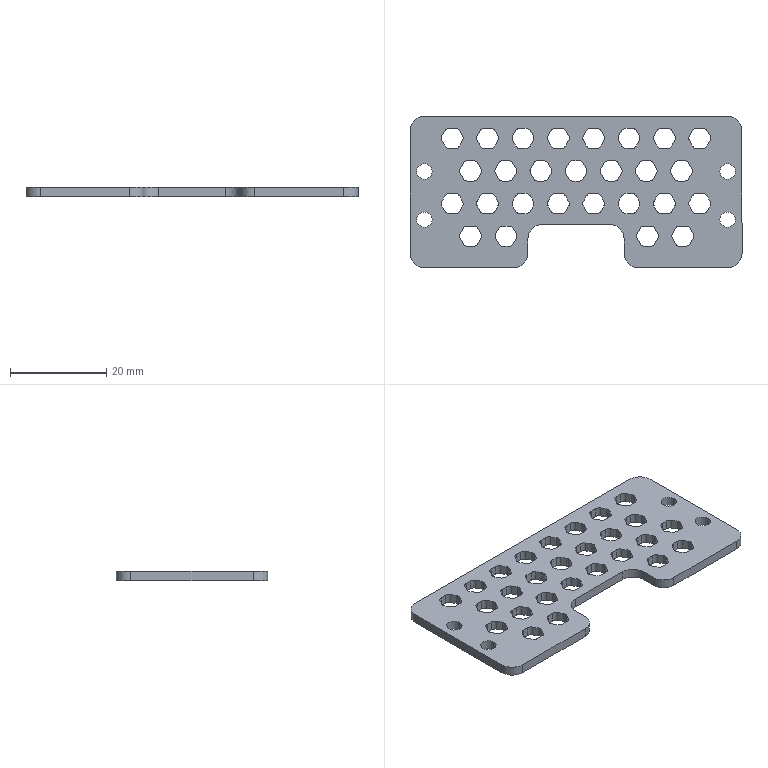Part | SolidWorks | features Fillet 2, Extrusion 1, ICE 1 | 1 solid | 377 faces | box 69 x 31.5 x 2 mm | volume 3100 mm3 | cylinder 205 | plane 172 | commonest cylinder face diameters 2 x189 3.2 x8 6 x8